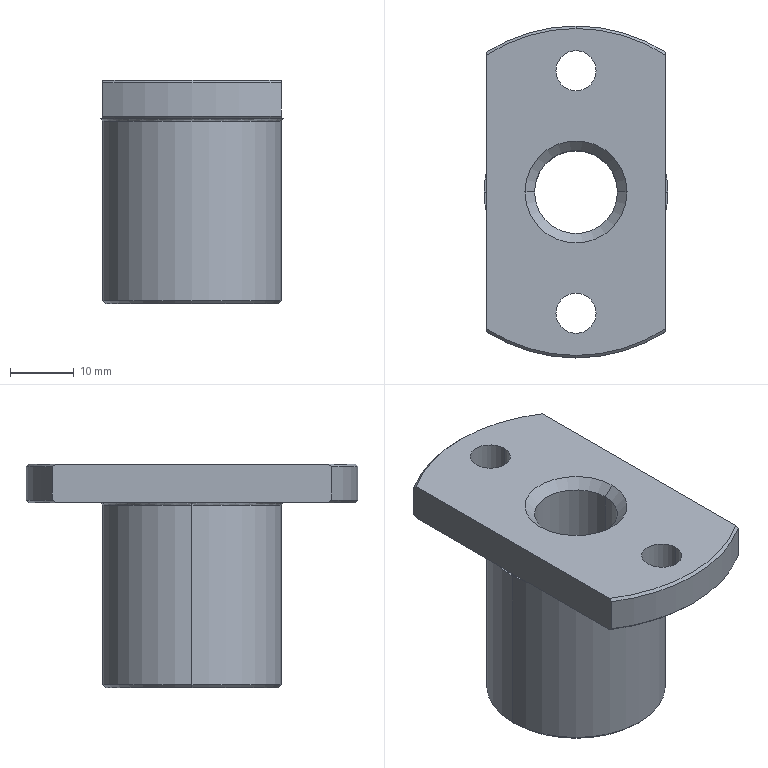Part | SolidWorks | features BaseBody 1 | 1 solid | 31 faces | box 28.8 x 52 x 35 mm | volume 21014 mm3 | cone 11 | cylinder 10 | plane 8 | spline 2 | commonest cylinder face diameters 6.3 x4 13 x2 28 x2 52 x2
STEP:
#1=CARTESIAN_POINT('',(14.4,0.,-6.));
#2=VERTEX_POINT('',#1);
#3=CARTESIAN_POINT('',(14.,3.37,-6.));
#4=VERTEX_POINT('',#3);
#5=CARTESIAN_POINT('',(14.4,0.,-6.));
#6=CARTESIAN_POINT('',(14.4,1.139,-6.));
#7=CARTESIAN_POINT('',(14.267,2.263,-6.));
#8=CARTESIAN_POINT('',(14.,3.37,-6.));
#9=B_SPLINE_CURVE_WITH_KNOTS('',3,(#5,#6,#7,#8),.UNSPECIFIED.,.F.,.F.,(4,4),(0.5,1.),.UNSPECIFIED.);
#10=EDGE_CURVE('',#2,#4,#9,.T.);
#11=ORIENTED_EDGE('',*,*,#10,.F.);
#12=CARTESIAN_POINT('',(14.,0.,-6.4));
#13=VERTEX_POINT('',#12);
#14=CARTESIAN_POINT('',(14.4,0.,-6.4));
#15=DIRECTION('',(0.,-1.,0.));
#16=DIRECTION('',(1.,0.,0.));
#17=AXIS2_PLACEMENT_3D('',#14,#15,#16);
#18=CIRCLE('',#17,0.4);
#19=EDGE_CURVE('',#2,#13,#18,.T.);
#20=ORIENTED_EDGE('',*,*,#19,.T.);
#21=CARTESIAN_POINT('',(-14.,0.,-6.4));
#22=VERTEX_POINT('',#21);
#23=CARTESIAN_POINT('',(0.,0.,-6.4));
#24=DIRECTION('',(0.,0.,-1.));
#25=DIRECTION('',(1.,0.,0.));
#26=AXIS2_PLACEMENT_3D('',#23,#24,#25);
#27=CIRCLE('',#26,14.);
#28=EDGE_CURVE('',#22,#13,#27,.T.);
#29=ORIENTED_EDGE('',*,*,#28,.F.);
#30=CARTESIAN_POINT('',(-14.4,0.,-6.));
#31=VERTEX_POINT('',#30);
#32=CARTESIAN_POINT('',(-14.4,0.,-6.4));
#33=DIRECTION('',(0.,1.,0.));
#34=DIRECTION('',(-1.,0.,0.));
#35=AXIS2_PLACEMENT_3D('',#32,#33,#34);
#36=CIRCLE('',#35,0.4);
#37=EDGE_CURVE('',#31,#22,#36,.T.);
#38=ORIENTED_EDGE('',*,*,#37,.F.);
#39=CARTESIAN_POINT('',(-14.,3.37,-6.));
#40=VERTEX_POINT('',#39);
#41=CARTESIAN_POINT('',(-14.,3.37,-6.));
#42=CARTESIAN_POINT('',(-14.267,2.262,-6.));
#43=CARTESIAN_POINT('',(-14.4,1.139,-6.));
#44=CARTESIAN_POINT('',(-14.4,0.,-6.));
#45=B_SPLINE_CURVE_WITH_KNOTS('',3,(#41,#42,#43,#44),.UNSPECIFIED.,.F.,.F.,(4,4),(0.,0.5),.UNSPECIFIED.);
#46=EDGE_CURVE('',#40,#31,#45,.T.);
#47=ORIENTED_EDGE('',*,*,#46,.F.);
#48=CARTESIAN_POINT('',(14.,3.37,-6.));
#49=CARTESIAN_POINT('',(13.911,3.742,-6.));
#50=CARTESIAN_POINT('',(13.755,4.291,-6.));
#51=CARTESIAN_POINT('',(13.536,4.92,-6.));
#52=CARTESIAN_POINT('',(13.417,5.231,-6.));
#53=CARTESIAN_POINT('',(13.364,5.363,-6.));
#54=CARTESIAN_POINT('',(13.328,5.452,-6.));
#55=CARTESIAN_POINT('',(13.311,5.494,-6.));
#56=CARTESIAN_POINT('',(13.139,5.907,-6.));
#57=CARTESIAN_POINT('',(12.887,6.447,-6.));
#58=CARTESIAN_POINT('',(12.555,7.057,-6.));
#59=CARTESIAN_POINT('',(12.38,7.357,-6.));
#60=CARTESIAN_POINT('',(12.302,7.484,-6.));
#61=CARTESIAN_POINT('',(12.251,7.569,-6.));
#62=CARTESIAN_POINT('',(12.225,7.61,-6.));
#63=CARTESIAN_POINT('',(11.98,8.,-6.));
#64=CARTESIAN_POINT('',(11.632,8.505,-6.));
#65=CARTESIAN_POINT('',(11.19,9.067,-6.));
#66=CARTESIAN_POINT('',(10.993,9.302,-6.));
#67=CARTESIAN_POINT('',(10.86,9.457,-6.));
#68=CARTESIAN_POINT('',(10.794,9.533,-6.));
#69=CARTESIAN_POINT('',(10.169,10.23,-6.));
#70=CARTESIAN_POINT('',(9.565,10.796,-6.));
#71=CARTESIAN_POINT('',(8.585,11.569,-6.));
#72=CARTESIAN_POINT('',(8.08,11.932,-6.));
#73=CARTESIAN_POINT('',(7.465,12.317,-6.));
#74=CARTESIAN_POINT('',(7.196,12.474,-6.));
#75=CARTESIAN_POINT('',(7.015,12.576,-6.));
#76=CARTESIAN_POINT('',(6.923,12.627,-6.));
#77=CARTESIAN_POINT('',(6.472,12.87,-6.));
#78=CARTESIAN_POINT('',(5.921,13.138,-6.));
#79=CARTESIAN_POINT('',(5.259,13.408,-6.));
#80=CARTESIAN_POINT('',(4.924,13.533,-6.));
#81=CARTESIAN_POINT('',(4.779,13.584,-6.));
#82=CARTESIAN_POINT('',(4.683,13.618,-6.));
#83=CARTESIAN_POINT('',(4.633,13.635,-6.));
#84=CARTESIAN_POINT('',(4.208,13.777,-6.));
#85=CARTESIAN_POINT('',(3.636,13.943,-6.));
#86=CARTESIAN_POINT('',(2.959,14.095,-6.));
#87=CARTESIAN_POINT('',(2.618,14.161,-6.));
#88=CARTESIAN_POINT('',(2.471,14.187,-6.));
#89=CARTESIAN_POINT('',(2.373,14.203,-6.));
#90=CARTESIAN_POINT('',(2.322,14.212,-6.));
#91=CARTESIAN_POINT('',(1.521,14.34,-6.));
#92=CARTESIAN_POINT('',(0.7634,14.4,-6.));
#93=CARTESIAN_POINT('',(-0.3817,14.4,-6.));
#94=CARTESIAN_POINT('',(-0.9524,14.377,-6.));
#95=CARTESIAN_POINT('',(-1.615,14.311,-6.));
#96=CARTESIAN_POINT('',(-1.945,14.269,-6.));
#97=CARTESIAN_POINT('',(-2.086,14.248,-6.));
#98=CARTESIAN_POINT('',(-2.181,14.234,-6.));
#99=CARTESIAN_POINT('',(-2.226,14.227,-6.));
#100=CARTESIAN_POINT('',(-2.668,14.156,-6.));
#101=CARTESIAN_POINT('',(-3.252,14.038,-6.));
#102=CARTESIAN_POINT('',(-3.922,13.858,-6.));
#103=CARTESIAN_POINT('',(-4.255,13.758,-6.));
#104=CARTESIAN_POINT('',(-4.397,13.712,-6.));
#105=CARTESIAN_POINT('',(-4.491,13.682,-6.));
#106=CARTESIAN_POINT('',(-4.537,13.667,-6.));
#107=CARTESIAN_POINT('',(-4.974,13.52,-6.));
#108=CARTESIAN_POINT('',(-5.547,13.3,-6.));
#109=CARTESIAN_POINT('',(-6.196,13.002,-6.));
#110=CARTESIAN_POINT('',(-6.47,12.865,-6.));
#111=CARTESIAN_POINT('',(-6.652,12.772,-6.));
#112=CARTESIAN_POINT('',(-6.741,12.725,-6.));
#113=CARTESIAN_POINT('',(-7.565,12.281,-6.));
#114=CARTESIAN_POINT('',(-8.258,11.826,-6.));
#115=CARTESIAN_POINT('',(-9.238,11.054,-6.));
#116=CARTESIAN_POINT('',(-9.71,10.648,-6.));
#117=CARTESIAN_POINT('',(-10.228,10.14,-6.));
#118=CARTESIAN_POINT('',(-10.443,9.916,-6.));
#119=CARTESIAN_POINT('',(-10.585,9.764,-6.));
#120=CARTESIAN_POINT('',(-10.656,9.686,-6.));
#121=CARTESIAN_POINT('',(-10.998,9.305,-6.));
#122=CARTESIAN_POINT('',(-11.387,8.831,-6.));
#123=CARTESIAN_POINT('',(-11.805,8.251,-6.));
#124=CARTESIAN_POINT('',(-12.004,7.955,-6.));
#125=CARTESIAN_POINT('',(-12.088,7.826,-6.));
#126=CARTESIAN_POINT('',(-12.143,7.74,-6.));
#127=CARTESIAN_POINT('',(-12.171,7.695,-6.));
#128=CARTESIAN_POINT('',(-12.409,7.316,-6.));
#129=CARTESIAN_POINT('',(-12.705,6.799,-6.));
#130=CARTESIAN_POINT('',(-13.011,6.176,-6.));
#131=CARTESIAN_POINT('',(-13.155,5.859,-6.));
#132=CARTESIAN_POINT('',(-13.214,5.723,-6.));
#133=CARTESIAN_POINT('',(-13.253,5.631,-6.));
#134=CARTESIAN_POINT('',(-13.273,5.584,-6.));
#135=CARTESIAN_POINT('',(-13.585,4.836,-6.));
#136=CARTESIAN_POINT('',(-13.821,4.112,-6.));
#137=CARTESIAN_POINT('',(-14.,3.37,-6.));
#138=B_SPLINE_CURVE_WITH_KNOTS('',3,(#48,#49,#50,#51,#52,#53,#54,#55,#56,#57,#58,#59,#60,#61,#62,#63,#64,#65,#66,#67,#68,#69,#70,#71,#72,#73,#74,#75,#76,#77,#78,#79,#80,#81,#82,#83,#84,#85,#86,#87,#88,#89,#90,#91,#92,#93,#94,#95,#96,#97,#98,#99,#100,#101,#102,#103,#104,#105,#106,#107,#108,#109,#110,#111,#112,#113,#114,#115,#116,#117,#118,#119,#120,#121,#122,#123,#124,#125,#126,#127,#128,#129,#130,#131,#132,#133,#134,#135,#136,#137),.UNSPECIFIED.,.F.,.F.,(4,1,1,1,2,2,1,1,1,2,2,1,1,2,2,2,1,1,2,2,1,1,1,2,2,1,1,1,2,2,2,1,1,1,2,2,1,1,1,2,2,1,1,2,2,2,1,1,2,2,1,1,1,2,2,1,1,1,2,2,4),(0.,0.03125,0.04688,0.05469,0.05859,0.0625,0.09375,0.1094,0.1172,0.1211,0.125,0.1563,0.1719,0.1797,0.1875,0.25,0.2813,0.2969,0.3047,0.3125,0.3438,0.3594,0.3672,0.3711,0.375,0.4063,0.4219,0.4297,0.4336,0.4375,0.5,0.5313,0.5469,0.5547,0.5586,0.5625,0.5938,0.6094,0.6172,0.6211,0.625,0.6563,0.6719,0.6797,0.6875,0.75,0.7813,0.7969,0.8047,0.8125,0.8438,0.8594,0.8672,0.8711,0.875,0.9063,0.9219,0.9297,0.9336,0.9375,1.),.UNSPECIFIED.);
#139=EDGE_CURVE('',#4,#40,#138,.T.);
#140=ORIENTED_EDGE('',*,*,#139,.F.);
#141=EDGE_LOOP('',(#11,#20,#29,#38,#47,#140));
#142=FACE_OUTER_BOUND('',#141,.T.);
#143=CARTESIAN_POINT('',(-14.4,0.,-6.));
#144=CARTESIAN_POINT('',(-14.4,28.8,-6.));
#145=CARTESIAN_POINT('',(14.4,28.8,-6.));
#146=CARTESIAN_POINT('',(14.4,0.,-6.));
#147=CARTESIAN_POINT('',(-14.166,0.,-6.));
#148=CARTESIAN_POINT('',(-14.166,28.331,-6.));
#149=CARTESIAN_POINT('',(14.166,28.331,-6.));
#150=CARTESIAN_POINT('',(14.166,0.,-6.));
#151=CARTESIAN_POINT('',(-14.,0.,-6.166));
#152=CARTESIAN_POINT('',(-14.,28.,-6.166));
#153=CARTESIAN_POINT('',(14.,28.,-6.166));
#154=CARTESIAN_POINT('',(14.,0.,-6.166));
#155=CARTESIAN_POINT('',(-14.,0.,-6.4));
#156=CARTESIAN_POINT('',(-14.,28.,-6.4));
#157=CARTESIAN_POINT('',(14.,28.,-6.4));
#158=CARTESIAN_POINT('',(14.,0.,-6.4));
#159=(BOUNDED_SURFACE()B_SPLINE_SURFACE(3,3,((#143,#144,#145,#146),(#147,#148,#149,#150),(#151,#152,#153,#154),(#155,#156,#157,#158)),.UNSPECIFIED.,.F.,.F.,.F.)B_SPLINE_SURFACE_WITH_KNOTS((4,4),(4,4),(0.,1.),(0.,1.),.UNSPECIFIED.)GEOMETRIC_REPRESENTATION_ITEM()RATIONAL_B_SPLINE_SURFACE(((1.,0.3333,0.3333,1.),(0.8047,0.2682,0.2682,0.8047),(0.8047,0.2682,0.2682,0.8047),(1.,0.3333,0.3333,1.)))REPRESENTATION_ITEM('')SURFACE());
#160=ADVANCED_FACE('',(#142),#159,.F.);
#161=CARTESIAN_POINT('',(14.,0.,-34.5));
#162=VERTEX_POINT('',#161);
#163=CARTESIAN_POINT('',(-14.,0.,-34.5));
#164=VERTEX_POINT('',#163);
#165=CARTESIAN_POINT('',(0.,0.,-34.5));
#166=DIRECTION('',(0.,0.,1.));
#167=DIRECTION('',(1.,0.,0.));
#168=AXIS2_PLACEMENT_3D('',#165,#166,#167);
#169=CIRCLE('',#168,14.);
#170=EDGE_CURVE('',#162,#164,#169,.T.);
#171=ORIENTED_EDGE('',*,*,#170,.T.);
#172=CARTESIAN_POINT('',(-14.,0.,-35.));
#173=DIRECTION('',(0.,0.,1.));
#174=VECTOR('',#173,1000.);
#175=LINE('',#172,#174);
#176=EDGE_CURVE('',#164,#22,#175,.T.);
#177=ORIENTED_EDGE('',*,*,#176,.T.);
#178=ORIENTED_EDGE('',*,*,#28,.T.);
#179=CARTESIAN_POINT('',(14.,0.,-35.));
#180=DIRECTION('',(0.,0.,1.));
#181=VECTOR('',#180,1000.);
#182=LINE('',#179,#181);
#183=EDGE_CURVE('',#162,#13,#182,.T.);
#184=ORIENTED_EDGE('',*,*,#183,.F.);
#185=EDGE_LOOP('',(#171,#177,#178,#184));
#186=FACE_OUTER_BOUND('',#185,.T.);
#187=CARTESIAN_POINT('',(0.,0.,-35.));
#188=DIRECTION('',(0.,0.,1.));
#189=DIRECTION('',(1.,0.,0.));
#190=AXIS2_PLACEMENT_3D('',#187,#188,#189);
#191=CYLINDRICAL_SURFACE('',#190,14.);
#192=ADVANCED_FACE('',(#186),#191,.T.);
#193=CARTESIAN_POINT('',(13.5,0.,-35.));
#194=VERTEX_POINT('',#193);
#195=CARTESIAN_POINT('',(-13.5,0.,-35.));
#196=VERTEX_POINT('',#195);
#197=CARTESIAN_POINT('',(0.,0.,-35.));
#198=DIRECTION('',(0.,0.,1.));
#199=DIRECTION('',(1.,0.,0.));
#200=AXIS2_PLACEMENT_3D('',#197,#198,#199);
#201=CIRCLE('',#200,13.5);
#202=EDGE_CURVE('',#194,#196,#201,.T.);
#203=ORIENTED_EDGE('',*,*,#202,.T.);
#204=CARTESIAN_POINT('',(-14.,0.,-34.5));
#205=DIRECTION('',(-0.7071,0.,0.7071));
#206=VECTOR('',#205,1000.);
#207=LINE('',#204,#206);
#208=EDGE_CURVE('',#196,#164,#207,.T.);
#209=ORIENTED_EDGE('',*,*,#208,.T.);
#210=ORIENTED_EDGE('',*,*,#170,.F.);
#211=CARTESIAN_POINT('',(14.,0.,-34.5));
#212=DIRECTION('',(0.7071,0.,0.7071));
#213=VECTOR('',#212,1000.);
#214=LINE('',#211,#213);
#215=EDGE_CURVE('',#194,#162,#214,.T.);
#216=ORIENTED_EDGE('',*,*,#215,.F.);
#217=EDGE_LOOP('',(#203,#209,#210,#216));
#218=FACE_OUTER_BOUND('',#217,.T.);
#219=CARTESIAN_POINT('',(0.,0.,-34.5));
#220=DIRECTION('',(0.,0.,1.));
#221=DIRECTION('',(1.,0.,0.));
#222=AXIS2_PLACEMENT_3D('',#219,#220,#221);
#223=CONICAL_SURFACE('',#222,14.,0.7854);
#224=ADVANCED_FACE('',(#218),#223,.T.);
#225=CARTESIAN_POINT('',(3.15,19.,0.));
#226=VERTEX_POINT('',#225);
#227=CARTESIAN_POINT('',(-3.15,19.,0.));
#228=VERTEX_POINT('',#227);
#229=CARTESIAN_POINT('',(0.,19.,0.));
#230=DIRECTION('',(0.,0.,-1.));
#231=DIRECTION('',(-1.,0.,0.));
#232=AXIS2_PLACEMENT_3D('',#229,#230,#231);
#233=CIRCLE('',#232,3.15);
#234=EDGE_CURVE('',#226,#228,#233,.T.);
#235=ORIENTED_EDGE('',*,*,#234,.F.);
#236=CARTESIAN_POINT('',(3.15,19.,-6.));
#237=VERTEX_POINT('',#236);
#238=CARTESIAN_POINT('',(3.15,19.,-6.));
#239=DIRECTION('',(0.,0.,-1.));
#240=VECTOR('',#239,1000.);
#241=LINE('',#238,#240);
#242=EDGE_CURVE('',#226,#237,#241,.T.);
#243=ORIENTED_EDGE('',*,*,#242,.T.);
#244=CARTESIAN_POINT('',(-3.15,19.,-6.));
#245=VERTEX_POINT('',#244);
#246=CARTESIAN_POINT('',(0.,19.,-6.));
#247=DIRECTION('',(0.,0.,-1.));
#248=DIRECTION('',(-1.,0.,0.));
#249=AXIS2_PLACEMENT_3D('',#246,#247,#248);
#250=CIRCLE('',#249,3.15);
#251=EDGE_CURVE('',#237,#245,#250,.T.);
#252=ORIENTED_EDGE('',*,*,#251,.T.);
#253=CARTESIAN_POINT('',(-3.15,19.,-6.));
#254=DIRECTION('',(0.,0.,-1.));
#255=VECTOR('',#254,1000.);
#256=LINE('',#253,#255);
#257=EDGE_CURVE('',#228,#245,#256,.T.);
#258=ORIENTED_EDGE('',*,*,#257,.F.);
#259=EDGE_LOOP('',(#235,#243,#252,#258));
#260=FACE_OUTER_BOUND('',#259,.T.);
#261=CARTESIAN_POINT('',(0.,19.,-6.));
#262=DIRECTION('',(0.,0.,-1.));
#263=DIRECTION('',(-1.,0.,0.));
#264=AXIS2_PLACEMENT_3D('',#261,#262,#263);
#265=CYLINDRICAL_SURFACE('',#264,3.15);
#266=ADVANCED_FACE('',(#260),#265,.F.);
#267=CARTESIAN_POINT('',(3.15,-19.,0.));
#268=VERTEX_POINT('',#267);
#269=CARTESIAN_POINT('',(-3.15,-19.,0.));
#270=VERTEX_POINT('',#269);
#271=CARTESIAN_POINT('',(0.,-19.,0.));
#272=DIRECTION('',(0.,0.,-1.));
#273=DIRECTION('',(-1.,0.,0.));
#274=AXIS2_PLACEMENT_3D('',#271,#272,#273);
#275=CIRCLE('',#274,3.15);
#276=EDGE_CURVE('',#268,#270,#275,.T.);
#277=ORIENTED_EDGE('',*,*,#276,.F.);
#278=CARTESIAN_POINT('',(3.15,-19.,-6.));
#279=VERTEX_POINT('',#278);
#280=CARTESIAN_POINT('',(3.15,-19.,-6.));
#281=DIRECTION('',(0.,0.,-1.));
#282=VECTOR('',#281,1000.);
#283=LINE('',#280,#282);
#284=EDGE_CURVE('',#268,#279,#283,.T.);
#285=ORIENTED_EDGE('',*,*,#284,.T.);
#286=CARTESIAN_POINT('',(-3.15,-19.,-6.));
#287=VERTEX_POINT('',#286);
#288=CARTESIAN_POINT('',(0.,-19.,-6.));
#289=DIRECTION('',(0.,0.,-1.));
#290=DIRECTION('',(-1.,0.,0.));
#291=AXIS2_PLACEMENT_3D('',#288,#289,#290);
#292=CIRCLE('',#291,3.15);
#293=EDGE_CURVE('',#279,#287,#292,.T.);
#294=ORIENTED_EDGE('',*,*,#293,.T.);
#295=CARTESIAN_POINT('',(-3.15,-19.,-6.));
#296=DIRECTION('',(0.,0.,-1.));
#297=VECTOR('',#296,1000.);
#298=LINE('',#295,#297);
#299=EDGE_CURVE('',#270,#287,#298,.T.);
#300=ORIENTED_EDGE('',*,*,#299,.F.);
#301=EDGE_LOOP('',(#277,#285,#294,#300));
#302=FACE_OUTER_BOUND('',#301,.T.);
#303=CARTESIAN_POINT('',(0.,-19.,-6.));
#304=DIRECTION('',(0.,0.,-1.));
#305=DIRECTION('',(-1.,0.,0.));
#306=AXIS2_PLACEMENT_3D('',#303,#304,#305);
#307=CYLINDRICAL_SURFACE('',#306,3.15);
#308=ADVANCED_FACE('',(#302),#307,.F.);
#309=CARTESIAN_POINT('',(6.5,0.,-33.5));
#310=VERTEX_POINT('',#309);
#311=CARTESIAN_POINT('',(-6.5,0.,-33.5));
#312=VERTEX_POINT('',#311);
#313=CARTESIAN_POINT('',(0.,0.,-33.5));
#314=DIRECTION('',(0.,0.,-1.));
#315=DIRECTION('',(-1.,0.,0.));
#316=AXIS2_PLACEMENT_3D('',#313,#314,#315);
#317=CIRCLE('',#316,6.5);
#318=EDGE_CURVE('',#310,#312,#317,.T.);
#319=ORIENTED_EDGE('',*,*,#318,.F.);
#320=CARTESIAN_POINT('',(8.,0.,-35.));
#321=VERTEX_POINT('',#320);
#322=CARTESIAN_POINT('',(8.,0.,-35.));
#323=DIRECTION('',(0.7071,0.,-0.7071));
#324=VECTOR('',#323,1000.);
#325=LINE('',#322,#324);
#326=EDGE_CURVE('',#310,#321,#325,.T.);
#327=ORIENTED_EDGE('',*,*,#326,.T.);
#328=CARTESIAN_POINT('',(-8.,0.,-35.));
#329=VERTEX_POINT('',#328);
#330=CARTESIAN_POINT('',(0.,0.,-35.));
#331=DIRECTION('',(0.,0.,-1.));
#332=DIRECTION('',(-1.,0.,0.));
#333=AXIS2_PLACEMENT_3D('',#330,#331,#332);
#334=CIRCLE('',#333,8.);
#335=EDGE_CURVE('',#321,#329,#334,.T.);
#336=ORIENTED_EDGE('',*,*,#335,.T.);
#337=CARTESIAN_POINT('',(-8.,0.,-35.));
#338=DIRECTION('',(-0.7071,0.,-0.7071));
#339=VECTOR('',#338,1000.);
#340=LINE('',#337,#339);
#341=EDGE_CURVE('',#312,#329,#340,.T.);
#342=ORIENTED_EDGE('',*,*,#341,.F.);
#343=EDGE_LOOP('',(#319,#327,#336,#342));
#344=FACE_OUTER_BOUND('',#343,.T.);
#345=CARTESIAN_POINT('',(0.,0.,-35.));
#346=DIRECTION('',(0.,0.,-1.));
#347=DIRECTION('',(-1.,0.,0.));
#348=AXIS2_PLACEMENT_3D('',#345,#346,#347);
#349=CONICAL_SURFACE('',#348,8.,0.7854);
#350=ADVANCED_FACE('',(#344),#349,.F.);
#351=ORIENTED_EDGE('',*,*,#318,.T.);
#352=CARTESIAN_POINT('',(-6.5,0.,-1.5));
#353=VERTEX_POINT('',#352);
#354=CARTESIAN_POINT('',(-6.5,0.,-35.));
#355=DIRECTION('',(0.,0.,1.));
#356=VECTOR('',#355,1000.);
#357=LINE('',#354,#356);
#358=EDGE_CURVE('',#312,#353,#357,.T.);
#359=ORIENTED_EDGE('',*,*,#358,.T.);
#360=CARTESIAN_POINT('',(6.5,0.,-1.5));
#361=VERTEX_POINT('',#360);
#362=CARTESIAN_POINT('',(0.,0.,-1.5));
#363=DIRECTION('',(0.,0.,-1.));
#364=DIRECTION('',(1.,0.,0.));
#365=AXIS2_PLACEMENT_3D('',#362,#363,#364);
#366=CIRCLE('',#365,6.5);
#367=EDGE_CURVE('',#361,#353,#366,.T.);
#368=ORIENTED_EDGE('',*,*,#367,.F.);
#369=CARTESIAN_POINT('',(6.5,0.,-35.));
#370=DIRECTION('',(0.,0.,1.));
#371=VECTOR('',#370,1000.);
#372=LINE('',#369,#371);
#373=EDGE_CURVE('',#310,#361,#372,.T.);
#374=ORIENTED_EDGE('',*,*,#373,.F.);
#375=EDGE_LOOP('',(#351,#359,#368,#374));
#376=FACE_OUTER_BOUND('',#375,.T.);
#377=CARTESIAN_POINT('',(0.,0.,-35.));
#378=DIRECTION('',(0.,0.,1.));
#379=DIRECTION('',(1.,0.,0.));
#380=AXIS2_PLACEMENT_3D('',#377,#378,#379);
#381=CYLINDRICAL_SURFACE('',#380,6.5);
#382=ADVANCED_FACE('',(#376),#381,.F.);
#383=ORIENTED_EDGE('',*,*,#367,.T.);
#384=CARTESIAN_POINT('',(-8.,0.,0.));
#385=VERTEX_POINT('',#384);
#386=CARTESIAN_POINT('',(-8.,0.,0.));
#387=DIRECTION('',(-0.7071,0.,0.7071));
#388=VECTOR('',#387,1000.);
#389=LINE('',#386,#388);
#390=EDGE_CURVE('',#353,#385,#389,.T.);
#391=ORIENTED_EDGE('',*,*,#390,.T.);
#392=CARTESIAN_POINT('',(8.,0.,0.));
#393=VERTEX_POINT('',#392);
#394=CARTESIAN_POINT('',(0.,0.,0.));
#395=DIRECTION('',(0.,0.,-1.));
#396=DIRECTION('',(1.,0.,0.));
#397=AXIS2_PLACEMENT_3D('',#394,#395,#396);
#398=CIRCLE('',#397,8.);
#399=EDGE_CURVE('',#393,#385,#398,.T.);
#400=ORIENTED_EDGE('',*,*,#399,.F.);
#401=CARTESIAN_POINT('',(8.,0.,0.));
#402=DIRECTION('',(0.7071,0.,0.7071));
#403=VECTOR('',#402,1000.);
#404=LINE('',#401,#403);
#405=EDGE_CURVE('',#361,#393,#404,.T.);
#406=ORIENTED_EDGE('',*,*,#405,.F.);
#407=EDGE_LOOP('',(#383,#391,#400,#406));
#408=FACE_OUTER_BOUND('',#407,.T.);
#409=CARTESIAN_POINT('',(0.,0.,0.));
#410=DIRECTION('',(0.,0.,1.));
#411=DIRECTION('',(1.,0.,0.));
#412=AXIS2_PLACEMENT_3D('',#409,#410,#411);
#413=CONICAL_SURFACE('',#412,8.,0.7854);
#414=ADVANCED_FACE('',(#408),#413,.F.);
#415=CARTESIAN_POINT('',(0.,25.6,0.));
#416=VERTEX_POINT('',#415);
#417=CARTESIAN_POINT('',(-14.,21.433,0.));
#418=VERTEX_POINT('',#417);
#419=CARTESIAN_POINT('',(0.,0.,0.));
#420=DIRECTION('',(0.,0.,1.));
#421=DIRECTION('',(0.,1.,0.));
#422=AXIS2_PLACEMENT_3D('',#419,#420,#421);
#423=CIRCLE('',#422,25.6);
#424=EDGE_CURVE('',#416,#418,#423,.T.);
#425=ORIENTED_EDGE('',*,*,#424,.F.);
#426=CARTESIAN_POINT('',(0.,26.,-0.4));
#427=VERTEX_POINT('',#426);
#428=CARTESIAN_POINT('',(0.,26.,-0.4));
#429=DIRECTION('',(0.,0.7071,-0.7071));
#430=VECTOR('',#429,1000.);
#431=LINE('',#428,#430);
#432=EDGE_CURVE('',#416,#427,#431,.T.);
#433=ORIENTED_EDGE('',*,*,#432,.T.);
#434=CARTESIAN_POINT('',(-14.,21.909,-0.4));
#435=VERTEX_POINT('',#434);
#436=CARTESIAN_POINT('',(0.,0.,-0.4));
#437=DIRECTION('',(0.,0.,-1.));
#438=DIRECTION('',(-1.,0.,0.));
#439=AXIS2_PLACEMENT_3D('',#436,#437,#438);
#440=CIRCLE('',#439,26.);
#441=EDGE_CURVE('',#435,#427,#440,.T.);
#442=ORIENTED_EDGE('',*,*,#441,.F.);
#443=CARTESIAN_POINT('',(-14.,21.909,-0.4));
#444=CARTESIAN_POINT('',(-14.,21.75,-0.2664));
#445=CARTESIAN_POINT('',(-14.,21.592,-0.1331));
#446=CARTESIAN_POINT('',(-14.,21.433,0.));
#447=B_SPLINE_CURVE_WITH_KNOTS('',3,(#443,#444,#445,#446),.UNSPECIFIED.,.F.,.F.,(4,4),(0.,0.0006219),.UNSPECIFIED.);
#448=EDGE_CURVE('',#435,#418,#447,.T.);
#449=ORIENTED_EDGE('',*,*,#448,.T.);
#450=EDGE_LOOP('',(#425,#433,#442,#449));
#451=FACE_OUTER_BOUND('',#450,.T.);
#452=CARTESIAN_POINT('',(0.,0.,-0.4));
#453=DIRECTION('',(0.,0.,-1.));
#454=DIRECTION('',(0.,1.,0.));
#455=AXIS2_PLACEMENT_3D('',#452,#453,#454);
#456=CONICAL_SURFACE('',#455,26.,0.7854);
#457=ADVANCED_FACE('',(#451),#456,.T.);
#458=ORIENTED_EDGE('',*,*,#176,.F.);
#459=CARTESIAN_POINT('',(0.,0.,-34.5));
#460=DIRECTION('',(0.,0.,1.));
#461=DIRECTION('',(1.,0.,0.));
#462=AXIS2_PLACEMENT_3D('',#459,#460,#461);
#463=CIRCLE('',#462,14.);
#464=EDGE_CURVE('',#164,#162,#463,.T.);
#465=ORIENTED_EDGE('',*,*,#464,.T.);
#466=ORIENTED_EDGE('',*,*,#183,.T.);
#467=CARTESIAN_POINT('',(0.,0.,-6.4));
#468=DIRECTION('',(0.,0.,-1.));
#469=DIRECTION('',(1.,0.,0.));
#470=AXIS2_PLACEMENT_3D('',#467,#468,#469);
#471=CIRCLE('',#470,14.);
#472=EDGE_CURVE('',#13,#22,#471,.T.);
#473=ORIENTED_EDGE('',*,*,#472,.T.);
#474=EDGE_LOOP('',(#458,#465,#466,#473));
#475=FACE_OUTER_BOUND('',#474,.T.);
#476=CARTESIAN_POINT('',(0.,0.,-35.));
#477=DIRECTION('',(0.,0.,1.));
#478=DIRECTION('',(1.,0.,0.));
#479=AXIS2_PLACEMENT_3D('',#476,#477,#478);
#480=CYLINDRICAL_SURFACE('',#479,14.);
#481=ADVANCED_FACE('',(#475),#480,.T.);
#482=ORIENTED_EDGE('',*,*,#19,.F.);
#483=CARTESIAN_POINT('',(14.,-3.37,-6.));
#484=VERTEX_POINT('',#483);
#485=CARTESIAN_POINT('',(14.,-3.37,-6.));
#486=CARTESIAN_POINT('',(14.267,-2.262,-6.));
#487=CARTESIAN_POINT('',(14.4,-1.139,-6.));
#488=CARTESIAN_POINT('',(14.4,0.,-6.));
#489=B_SPLINE_CURVE_WITH_KNOTS('',3,(#485,#486,#487,#488),.UNSPECIFIED.,.F.,.F.,(4,4),(0.,0.5),.UNSPECIFIED.);
#490=EDGE_CURVE('',#484,#2,#489,.T.);
#491=ORIENTED_EDGE('',*,*,#490,.F.);
#492=CARTESIAN_POINT('',(-14.,-3.37,-6.));
#493=VERTEX_POINT('',#492);
#494=CARTESIAN_POINT('',(-14.,-3.37,-6.));
#495=CARTESIAN_POINT('',(-13.911,-3.742,-6.));
#496=CARTESIAN_POINT('',(-13.755,-4.291,-6.));
#497=CARTESIAN_POINT('',(-13.536,-4.92,-6.));
#498=CARTESIAN_POINT('',(-13.417,-5.231,-6.));
#499=CARTESIAN_POINT('',(-13.364,-5.363,-6.));
#500=CARTESIAN_POINT('',(-13.328,-5.452,-6.));
#501=CARTESIAN_POINT('',(-13.311,-5.494,-6.));
#502=CARTESIAN_POINT('',(-13.139,-5.907,-6.));
#503=CARTESIAN_POINT('',(-12.887,-6.447,-6.));
#504=CARTESIAN_POINT('',(-12.555,-7.057,-6.));
#505=CARTESIAN_POINT('',(-12.38,-7.357,-6.));
#506=CARTESIAN_POINT('',(-12.302,-7.484,-6.));
#507=CARTESIAN_POINT('',(-12.251,-7.569,-6.));
#508=CARTESIAN_POINT('',(-12.225,-7.61,-6.));
#509=CARTESIAN_POINT('',(-11.98,-8.,-6.));
#510=CARTESIAN_POINT('',(-11.632,-8.505,-6.));
#511=CARTESIAN_POINT('',(-11.19,-9.067,-6.));
#512=CARTESIAN_POINT('',(-10.993,-9.302,-6.));
#513=CARTESIAN_POINT('',(-10.86,-9.457,-6.));
#514=CARTESIAN_POINT('',(-10.794,-9.533,-6.));
#515=CARTESIAN_POINT('',(-10.169,-10.23,-6.));
#516=CARTESIAN_POINT('',(-9.565,-10.796,-6.));
#517=CARTESIAN_POINT('',(-8.585,-11.569,-6.));
#518=CARTESIAN_POINT('',(-8.08,-11.932,-6.));
#519=CARTESIAN_POINT('',(-7.465,-12.317,-6.));
#520=CARTESIAN_POINT('',(-7.196,-12.474,-6.));
#521=CARTESIAN_POINT('',(-7.015,-12.576,-6.));
#522=CARTESIAN_POINT('',(-6.923,-12.627,-6.));
#523=CARTESIAN_POINT('',(-6.472,-12.87,-6.));
#524=CARTESIAN_POINT('',(-5.921,-13.138,-6.));
#525=CARTESIAN_POINT('',(-5.259,-13.408,-6.));
#526=CARTESIAN_POINT('',(-4.924,-13.533,-6.));
#527=CARTESIAN_POINT('',(-4.779,-13.584,-6.));
#528=CARTESIAN_POINT('',(-4.683,-13.618,-6.));
#529=CARTESIAN_POINT('',(-4.633,-13.635,-6.));
#530=CARTESIAN_POINT('',(-4.208,-13.777,-6.));
#531=CARTESIAN_POINT('',(-3.636,-13.943,-6.));
#532=CARTESIAN_POINT('',(-2.959,-14.095,-6.));
#533=CARTESIAN_POINT('',(-2.618,-14.161,-6.));
#534=CARTESIAN_POINT('',(-2.471,-14.187,-6.));
#535=CARTESIAN_POINT('',(-2.373,-14.203,-6.));
#536=CARTESIAN_POINT('',(-2.322,-14.212,-6.));
#537=CARTESIAN_POINT('',(-1.521,-14.34,-6.));
#538=CARTESIAN_POINT('',(-0.7634,-14.4,-6.));
#539=CARTESIAN_POINT('',(0.3817,-14.4,-6.));
#540=CARTESIAN_POINT('',(0.9524,-14.377,-6.));
#541=CARTESIAN_POINT('',(1.615,-14.311,-6.));
#542=CARTESIAN_POINT('',(1.945,-14.269,-6.));
#543=CARTESIAN_POINT('',(2.086,-14.248,-6.));
#544=CARTESIAN_POINT('',(2.181,-14.234,-6.));
#545=CARTESIAN_POINT('',(2.226,-14.227,-6.));
#546=CARTESIAN_POINT('',(2.668,-14.156,-6.));
#547=CARTESIAN_POINT('',(3.252,-14.038,-6.));
#548=CARTESIAN_POINT('',(3.922,-13.858,-6.));
#549=CARTESIAN_POINT('',(4.255,-13.758,-6.));
#550=CARTESIAN_POINT('',(4.397,-13.712,-6.));
#551=CARTESIAN_POINT('',(4.491,-13.682,-6.));
#552=CARTESIAN_POINT('',(4.537,-13.667,-6.));
#553=CARTESIAN_POINT('',(4.974,-13.52,-6.));
#554=CARTESIAN_POINT('',(5.547,-13.3,-6.));
#555=CARTESIAN_POINT('',(6.196,-13.002,-6.));
#556=CARTESIAN_POINT('',(6.47,-12.865,-6.));
#557=CARTESIAN_POINT('',(6.652,-12.772,-6.));
#558=CARTESIAN_POINT('',(6.741,-12.725,-6.));
#559=CARTESIAN_POINT('',(7.565,-12.281,-6.));
#560=CARTESIAN_POINT('',(8.258,-11.826,-6.));
#561=CARTESIAN_POINT('',(9.238,-11.054,-6.));
#562=CARTESIAN_POINT('',(9.71,-10.648,-6.));
#563=CARTESIAN_POINT('',(10.228,-10.14,-6.));
#564=CARTESIAN_POINT('',(10.443,-9.916,-6.));
#565=CARTESIAN_POINT('',(10.585,-9.764,-6.));
#566=CARTESIAN_POINT('',(10.656,-9.686,-6.));
#567=CARTESIAN_POINT('',(10.998,-9.305,-6.));
#568=CARTESIAN_POINT('',(11.387,-8.831,-6.));
#569=CARTESIAN_POINT('',(11.805,-8.251,-6.));
#570=CARTESIAN_POINT('',(12.004,-7.955,-6.));
#571=CARTESIAN_POINT('',(12.088,-7.826,-6.));
#572=CARTESIAN_POINT('',(12.143,-7.74,-6.));
#573=CARTESIAN_POINT('',(12.171,-7.695,-6.));
#574=CARTESIAN_POINT('',(12.409,-7.316,-6.));
#575=CARTESIAN_POINT('',(12.705,-6.799,-6.));
#576=CARTESIAN_POINT('',(13.011,-6.176,-6.));
#577=CARTESIAN_POINT('',(13.155,-5.859,-6.));
#578=CARTESIAN_POINT('',(13.214,-5.723,-6.));
#579=CARTESIAN_POINT('',(13.253,-5.631,-6.));
#580=CARTESIAN_POINT('',(13.273,-5.584,-6.));
#581=CARTESIAN_POINT('',(13.585,-4.836,-6.));
#582=CARTESIAN_POINT('',(13.821,-4.112,-6.));
#583=CARTESIAN_POINT('',(14.,-3.37,-6.));
#584=B_SPLINE_CURVE_WITH_KNOTS('',3,(#494,#495,#496,#497,#498,#499,#500,#501,#502,#503,#504,#505,#506,#507,#508,#509,#510,#511,#512,#513,#514,#515,#516,#517,#518,#519,#520,#521,#522,#523,#524,#525,#526,#527,#528,#529,#530,#531,#532,#533,#534,#535,#536,#537,#538,#539,#540,#541,#542,#543,#544,#545,#546,#547,#548,#549,#550,#551,#552,#553,#554,#555,#556,#557,#558,#559,#560,#561,#562,#563,#564,#565,#566,#567,#568,#569,#570,#571,#572,#573,#574,#575,#576,#577,#578,#579,#580,#581,#582,#583),.UNSPECIFIED.,.F.,.F.,(4,1,1,1,2,2,1,1,1,2,2,1,1,2,2,2,1,1,2,2,1,1,1,2,2,1,1,1,2,2,2,1,1,1,2,2,1,1,1,2,2,1,1,2,2,2,1,1,2,2,1,1,1,2,2,1,1,1,2,2,4),(0.,0.03125,0.04687,0.05469,0.05859,0.0625,0.09375,0.1094,0.1172,0.1211,0.125,0.1562,0.1719,0.1797,0.1875,0.25,0.2812,0.2969,0.3047,0.3125,0.3437,0.3594,0.3672,0.3711,0.375,0.4062,0.4219,0.4297,0.4336,0.4375,0.5,0.5313,0.5469,0.5547,0.5586,0.5625,0.5938,0.6094,0.6172,0.6211,0.625,0.6563,0.6719,0.6797,0.6875,0.75,0.7813,0.7969,0.8047,0.8125,0.8438,0.8594,0.8672,0.8711,0.875,0.9063,0.9219,0.9297,0.9336,0.9375,1.),.UNSPECIFIED.);
#585=EDGE_CURVE('',#493,#484,#584,.T.);
#586=ORIENTED_EDGE('',*,*,#585,.F.);
#587=CARTESIAN_POINT('',(-14.4,0.,-6.));
#588=CARTESIAN_POINT('',(-14.4,-1.139,-6.));
#589=CARTESIAN_POINT('',(-14.267,-2.263,-6.));
#590=CARTESIAN_POINT('',(-14.,-3.37,-6.));
#591=B_SPLINE_CURVE_WITH_KNOTS('',3,(#587,#588,#589,#590),.UNSPECIFIED.,.F.,.F.,(4,4),(0.5,1.),.UNSPECIFIED.);
#592=EDGE_CURVE('',#31,#493,#591,.T.);
#593=ORIENTED_EDGE('',*,*,#592,.F.);
#594=ORIENTED_EDGE('',*,*,#37,.T.);
#595=ORIENTED_EDGE('',*,*,#472,.F.);
#596=EDGE_LOOP('',(#482,#491,#586,#593,#594,#595));
#597=FACE_OUTER_BOUND('',#596,.T.);
#598=CARTESIAN_POINT('',(14.4,0.,-6.));
#599=CARTESIAN_POINT('',(14.4,-28.8,-6.));
#600=CARTESIAN_POINT('',(-14.4,-28.8,-6.));
#601=CARTESIAN_POINT('',(-14.4,0.,-6.));
#602=CARTESIAN_POINT('',(14.166,0.,-6.));
#603=CARTESIAN_POINT('',(14.166,-28.331,-6.));
#604=CARTESIAN_POINT('',(-14.166,-28.331,-6.));
#605=CARTESIAN_POINT('',(-14.166,0.,-6.));
#606=CARTESIAN_POINT('',(14.,0.,-6.166));
#607=CARTESIAN_POINT('',(14.,-28.,-6.166));
#608=CARTESIAN_POINT('',(-14.,-28.,-6.166));
#609=CARTESIAN_POINT('',(-14.,0.,-6.166));
#610=CARTESIAN_POINT('',(14.,0.,-6.4));
#611=CARTESIAN_POINT('',(14.,-28.,-6.4));
#612=CARTESIAN_POINT('',(-14.,-28.,-6.4));
#613=CARTESIAN_POINT('',(-14.,0.,-6.4));
#614=(BOUNDED_SURFACE()B_SPLINE_SURFACE(3,3,((#598,#599,#600,#601),(#602,#603,#604,#605),(#606,#607,#608,#609),(#610,#611,#612,#613)),.UNSPECIFIED.,.F.,.F.,.F.)B_SPLINE_SURFACE_WITH_KNOTS((4,4),(4,4),(0.,1.),(0.,1.),.UNSPECIFIED.)GEOMETRIC_REPRESENTATION_ITEM()RATIONAL_B_SPLINE_SURFACE(((1.,0.3333,0.3333,1.),(0.8047,0.2682,0.2682,0.8047),(0.8047,0.2682,0.2682,0.8047),(1.,0.3333,0.3333,1.)))REPRESENTATION_ITEM('')SURFACE());
#615=ADVANCED_FACE('',(#597),#614,.F.);
#616=ORIENTED_EDGE('',*,*,#208,.F.);
#617=CARTESIAN_POINT('',(0.,0.,-35.));
#618=DIRECTION('',(0.,0.,1.));
#619=DIRECTION('',(1.,0.,0.));
#620=AXIS2_PLACEMENT_3D('',#617,#618,#619);
#621=CIRCLE('',#620,13.5);
#622=EDGE_CURVE('',#196,#194,#621,.T.);
#623=ORIENTED_EDGE('',*,*,#622,.T.);
#624=ORIENTED_EDGE('',*,*,#215,.T.);
#625=ORIENTED_EDGE('',*,*,#464,.F.);
#626=EDGE_LOOP('',(#616,#623,#624,#625));
#627=FACE_OUTER_BOUND('',#626,.T.);
#628=CARTESIAN_POINT('',(0.,0.,-34.5));
#629=DIRECTION('',(0.,0.,1.));
#630=DIRECTION('',(1.,0.,0.));
#631=AXIS2_PLACEMENT_3D('',#628,#629,#630);
#632=CONICAL_SURFACE('',#631,14.,0.7854);
#633=ADVANCED_FACE('',(#627),#632,.T.);
#634=CARTESIAN_POINT('',(-14.,0.,-6.));
#635=DIRECTION('',(0.,-1.,0.));
#636=VECTOR('',#635,1000.);
#637=LINE('',#634,#636);
#638=EDGE_CURVE('',#40,#493,#637,.T.);
#639=ORIENTED_EDGE('',*,*,#638,.F.);
#640=ORIENTED_EDGE('',*,*,#46,.T.);
#641=ORIENTED_EDGE('',*,*,#592,.T.);
#642=EDGE_LOOP('',(#639,#640,#641));
#643=FACE_OUTER_BOUND('',#642,.T.);
#644=CARTESIAN_POINT('',(0.,0.,-6.));
#645=DIRECTION('',(0.,0.,-1.));
#646=DIRECTION('',(-1.,0.,0.));
#647=AXIS2_PLACEMENT_3D('',#644,#645,#646);
#648=PLANE('',#647);
#649=ADVANCED_FACE('',(#643),#648,.F.);
#650=CARTESIAN_POINT('',(14.,21.433,-6.));
#651=VERTEX_POINT('',#650);
#652=CARTESIAN_POINT('',(14.,0.,-6.));
#653=DIRECTION('',(0.,1.,0.));
#654=VECTOR('',#653,1000.);
#655=LINE('',#652,#654);
#656=EDGE_CURVE('',#4,#651,#655,.T.);
#657=ORIENTED_EDGE('',*,*,#656,.F.);
#658=ORIENTED_EDGE('',*,*,#139,.T.);
#659=CARTESIAN_POINT('',(-14.,21.433,-6.));
#660=VERTEX_POINT('',#659);
#661=CARTESIAN_POINT('',(-14.,0.,-6.));
#662=DIRECTION('',(0.,-1.,0.));
#663=VECTOR('',#662,1000.);
#664=LINE('',#661,#663);
#665=EDGE_CURVE('',#660,#40,#664,.T.);
#666=ORIENTED_EDGE('',*,*,#665,.F.);
#667=CARTESIAN_POINT('',(0.,0.,-6.));
#668=DIRECTION('',(0.,0.,1.));
#669=DIRECTION('',(1.,0.,0.));
#670=AXIS2_PLACEMENT_3D('',#667,#668,#669);
#671=CIRCLE('',#670,25.6);
#672=EDGE_CURVE('',#651,#660,#671,.T.);
#673=ORIENTED_EDGE('',*,*,#672,.F.);
#674=EDGE_LOOP('',(#657,#658,#666,#673));
#675=FACE_OUTER_BOUND('',#674,.T.);
#676=CARTESIAN_POINT('',(0.,19.,-6.));
#677=DIRECTION('',(0.,0.,-1.));
#678=DIRECTION('',(-1.,0.,0.));
#679=AXIS2_PLACEMENT_3D('',#676,#677,#678);
#680=CIRCLE('',#679,3.15);
#681=EDGE_CURVE('',#245,#237,#680,.T.);
#682=ORIENTED_EDGE('',*,*,#681,.F.);
#683=ORIENTED_EDGE('',*,*,#251,.F.);
#684=EDGE_LOOP('',(#682,#683));
#685=FACE_BOUND('',#684,.T.);
#686=CARTESIAN_POINT('',(0.,0.,-6.));
#687=DIRECTION('',(0.,0.,1.));
#688=DIRECTION('',(1.,0.,0.));
#689=AXIS2_PLACEMENT_3D('',#686,#687,#688);
#690=PLANE('',#689);
#691=ADVANCED_FACE('',(#675,#685),#690,.F.);
#692=CARTESIAN_POINT('',(14.,0.,-6.));
#693=DIRECTION('',(0.,1.,0.));
#694=VECTOR('',#693,1000.);
#695=LINE('',#692,#694);
#696=EDGE_CURVE('',#484,#4,#695,.T.);
#697=ORIENTED_EDGE('',*,*,#696,.F.);
#698=ORIENTED_EDGE('',*,*,#490,.T.);
#699=ORIENTED_EDGE('',*,*,#10,.T.);
#700=EDGE_LOOP('',(#697,#698,#699));
#701=FACE_OUTER_BOUND('',#700,.T.);
#702=CARTESIAN_POINT('',(0.,0.,-6.));
#703=DIRECTION('',(0.,0.,-1.));
#704=DIRECTION('',(-1.,0.,0.));
#705=AXIS2_PLACEMENT_3D('',#702,#703,#704);
#706=PLANE('',#705);
#707=ADVANCED_FACE('',(#701),#706,.F.);
#708=CARTESIAN_POINT('',(-14.,-21.433,-6.));
#709=VERTEX_POINT('',#708);
#710=CARTESIAN_POINT('',(14.,-21.433,-6.));
#711=VERTEX_POINT('',#710);
#712=CARTESIAN_POINT('',(0.,0.,-6.));
#713=DIRECTION('',(0.,0.,1.));
#714=DIRECTION('',(1.,0.,0.));
#715=AXIS2_PLACEMENT_3D('',#712,#713,#714);
#716=CIRCLE('',#715,25.6);
#717=EDGE_CURVE('',#709,#711,#716,.T.);
#718=ORIENTED_EDGE('',*,*,#717,.F.);
#719=CARTESIAN_POINT('',(-14.,0.,-6.));
#720=DIRECTION('',(0.,-1.,0.));
#721=VECTOR('',#720,1000.);
#722=LINE('',#719,#721);
#723=EDGE_CURVE('',#493,#709,#722,.T.);
#724=ORIENTED_EDGE('',*,*,#723,.F.);
#725=ORIENTED_EDGE('',*,*,#585,.T.);
#726=CARTESIAN_POINT('',(14.,0.,-6.));
#727=DIRECTION('',(0.,1.,0.));
#728=VECTOR('',#727,1000.);
#729=LINE('',#726,#728);
#730=EDGE_CURVE('',#711,#484,#729,.T.);
#731=ORIENTED_EDGE('',*,*,#730,.F.);
#732=EDGE_LOOP('',(#718,#724,#725,#731));
#733=FACE_OUTER_BOUND('',#732,.T.);
#734=CARTESIAN_POINT('',(0.,-19.,-6.));
#735=DIRECTION('',(0.,0.,-1.));
#736=DIRECTION('',(-1.,0.,0.));
#737=AXIS2_PLACEMENT_3D('',#734,#735,#736);
#738=CIRCLE('',#737,3.15);
#739=EDGE_CURVE('',#287,#279,#738,.T.);
#740=ORIENTED_EDGE('',*,*,#739,.F.);
#741=ORIENTED_EDGE('',*,*,#293,.F.);
#742=EDGE_LOOP('',(#740,#741));
#743=FACE_BOUND('',#742,.T.);
#744=CARTESIAN_POINT('',(0.,0.,-6.));
#745=DIRECTION('',(0.,0.,1.));
#746=DIRECTION('',(1.,0.,0.));
#747=AXIS2_PLACEMENT_3D('',#744,#745,#746);
#748=PLANE('',#747);
#749=ADVANCED_FACE('',(#733,#743),#748,.F.);
#750=ORIENTED_EDGE('',*,*,#202,.F.);
#751=ORIENTED_EDGE('',*,*,#622,.F.);
#752=EDGE_LOOP('',(#750,#751));
#753=FACE_OUTER_BOUND('',#752,.T.);
#754=CARTESIAN_POINT('',(0.,0.,-35.));
#755=DIRECTION('',(0.,0.,-1.));
#756=DIRECTION('',(-1.,0.,0.));
#757=AXIS2_PLACEMENT_3D('',#754,#755,#756);
#758=CIRCLE('',#757,8.);
#759=EDGE_CURVE('',#329,#321,#758,.T.);
#760=ORIENTED_EDGE('',*,*,#759,.F.);
#761=ORIENTED_EDGE('',*,*,#335,.F.);
#762=EDGE_LOOP('',(#760,#761));
#763=FACE_BOUND('',#762,.T.);
#764=CARTESIAN_POINT('',(0.,13.5,-35.));
#765=DIRECTION('',(0.,0.,1.));
#766=DIRECTION('',(1.,0.,0.));
#767=AXIS2_PLACEMENT_3D('',#764,#765,#766);
#768=PLANE('',#767);
#769=ADVANCED_FACE('',(#753,#763),#768,.F.);
#770=CARTESIAN_POINT('',(-14.,-21.433,0.));
#771=VERTEX_POINT('',#770);
#772=CARTESIAN_POINT('',(-14.,-21.909,-0.4));
#773=VERTEX_POINT('',#772);
#774=CARTESIAN_POINT('',(-14.,-21.433,0.));
#775=CARTESIAN_POINT('',(-14.,-21.592,-0.1331));
#776=CARTESIAN_POINT('',(-14.,-21.75,-0.2664));
#777=CARTESIAN_POINT('',(-14.,-21.909,-0.4));
#778=B_SPLINE_CURVE_WITH_KNOTS('',3,(#774,#775,#776,#777),.UNSPECIFIED.,.F.,.F.,(4,4),(0.,0.0006219),.UNSPECIFIED.);
#779=EDGE_CURVE('',#771,#773,#778,.T.);
#780=ORIENTED_EDGE('',*,*,#779,.F.);
#781=CARTESIAN_POINT('',(-14.,21.909,0.));
#782=DIRECTION('',(0.,1.,0.));
#783=VECTOR('',#782,1000.);
#784=LINE('',#781,#783);
#785=EDGE_CURVE('',#771,#418,#784,.T.);
#786=ORIENTED_EDGE('',*,*,#785,.T.);
#787=ORIENTED_EDGE('',*,*,#448,.F.);
#788=CARTESIAN_POINT('',(-14.,21.909,-5.6));
#789=VERTEX_POINT('',#788);
#790=CARTESIAN_POINT('',(-14.,21.909,-6.));
#791=DIRECTION('',(0.,0.,-1.));
#792=VECTOR('',#791,1000.);
#793=LINE('',#790,#792);
#794=EDGE_CURVE('',#435,#789,#793,.T.);
#795=ORIENTED_EDGE('',*,*,#794,.T.);
#796=CARTESIAN_POINT('',(-14.,21.909,-5.6));
#797=CARTESIAN_POINT('',(-14.,21.75,-5.734));
#798=CARTESIAN_POINT('',(-14.,21.592,-5.867));
#799=CARTESIAN_POINT('',(-14.,21.433,-6.));
#800=B_SPLINE_CURVE_WITH_KNOTS('',3,(#796,#797,#798,#799),.UNSPECIFIED.,.F.,.F.,(4,4),(0.,0.0006219),.UNSPECIFIED.);
#801=EDGE_CURVE('',#789,#660,#800,.T.);
#802=ORIENTED_EDGE('',*,*,#801,.T.);
#803=ORIENTED_EDGE('',*,*,#665,.T.);
#804=ORIENTED_EDGE('',*,*,#638,.T.);
#805=ORIENTED_EDGE('',*,*,#723,.T.);
#806=CARTESIAN_POINT('',(-14.,-21.909,-5.6));
#807=VERTEX_POINT('',#806);
#808=CARTESIAN_POINT('',(-14.,-21.433,-6.));
#809=CARTESIAN_POINT('',(-14.,-21.592,-5.867));
#810=CARTESIAN_POINT('',(-14.,-21.75,-5.734));
#811=CARTESIAN_POINT('',(-14.,-21.909,-5.6));
#812=B_SPLINE_CURVE_WITH_KNOTS('',3,(#808,#809,#810,#811),.UNSPECIFIED.,.F.,.F.,(4,4),(0.,0.0006219),.UNSPECIFIED.);
#813=EDGE_CURVE('',#709,#807,#812,.T.);
#814=ORIENTED_EDGE('',*,*,#813,.T.);
#815=CARTESIAN_POINT('',(-14.,-21.909,-6.));
#816=DIRECTION('',(0.,0.,1.));
#817=VECTOR('',#816,1000.);
#818=LINE('',#815,#817);
#819=EDGE_CURVE('',#807,#773,#818,.T.);
#820=ORIENTED_EDGE('',*,*,#819,.T.);
#821=EDGE_LOOP('',(#780,#786,#787,#795,#802,#803,#804,#805,#814,#820));
#822=FACE_OUTER_BOUND('',#821,.T.);
#823=CARTESIAN_POINT('',(-14.,21.909,-6.));
#824=DIRECTION('',(-1.,0.,0.));
#825=DIRECTION('',(0.,0.,1.));
#826=AXIS2_PLACEMENT_3D('',#823,#824,#825);
#827=PLANE('',#826);
#828=ADVANCED_FACE('',(#822),#827,.T.);
#829=CARTESIAN_POINT('',(14.,21.909,-5.6));
#830=VERTEX_POINT('',#829);
#831=CARTESIAN_POINT('',(14.,21.909,-5.6));
#832=CARTESIAN_POINT('',(14.,21.75,-5.734));
#833=CARTESIAN_POINT('',(14.,21.592,-5.867));
#834=CARTESIAN_POINT('',(14.,21.433,-6.));
#835=B_SPLINE_CURVE_WITH_KNOTS('',3,(#831,#832,#833,#834),.UNSPECIFIED.,.F.,.F.,(4,4),(0.,0.0006219),.UNSPECIFIED.);
#836=EDGE_CURVE('',#830,#651,#835,.T.);
#837=ORIENTED_EDGE('',*,*,#836,.T.);
#838=ORIENTED_EDGE('',*,*,#672,.T.);
#839=ORIENTED_EDGE('',*,*,#801,.F.);
#840=CARTESIAN_POINT('',(0.,0.,-5.6));
#841=DIRECTION('',(0.,0.,-1.));
#842=DIRECTION('',(1.,0.,0.));
#843=AXIS2_PLACEMENT_3D('',#840,#841,#842);
#844=CIRCLE('',#843,26.);
#845=EDGE_CURVE('',#789,#830,#844,.T.);
#846=ORIENTED_EDGE('',*,*,#845,.T.);
#847=EDGE_LOOP('',(#837,#838,#839,#846));
#848=FACE_OUTER_BOUND('',#847,.T.);
#849=CARTESIAN_POINT('',(0.,0.,-5.6));
#850=DIRECTION('',(0.,0.,1.));
#851=DIRECTION('',(1.,0.,0.));
#852=AXIS2_PLACEMENT_3D('',#849,#850,#851);
#853=CONICAL_SURFACE('',#852,26.,0.7854);
#854=ADVANCED_FACE('',(#848),#853,.T.);
#855=CARTESIAN_POINT('',(14.,21.433,0.));
#856=VERTEX_POINT('',#855);
#857=CARTESIAN_POINT('',(14.,21.909,-0.4));
#858=VERTEX_POINT('',#857);
#859=CARTESIAN_POINT('',(14.,21.433,0.));
#860=CARTESIAN_POINT('',(14.,21.592,-0.1331));
#861=CARTESIAN_POINT('',(14.,21.75,-0.2664));
#862=CARTESIAN_POINT('',(14.,21.909,-0.4));
#863=B_SPLINE_CURVE_WITH_KNOTS('',3,(#859,#860,#861,#862),.UNSPECIFIED.,.F.,.F.,(4,4),(0.,0.0006219),.UNSPECIFIED.);
#864=EDGE_CURVE('',#856,#858,#863,.T.);
#865=ORIENTED_EDGE('',*,*,#864,.F.);
#866=CARTESIAN_POINT('',(14.,-21.433,0.));
#867=VERTEX_POINT('',#866);
#868=CARTESIAN_POINT('',(14.,-21.909,0.));
#869=DIRECTION('',(0.,-1.,0.));
#870=VECTOR('',#869,1000.);
#871=LINE('',#868,#870);
#872=EDGE_CURVE('',#856,#867,#871,.T.);
#873=ORIENTED_EDGE('',*,*,#872,.T.);
#874=CARTESIAN_POINT('',(14.,-21.909,-0.4));
#875=VERTEX_POINT('',#874);
#876=CARTESIAN_POINT('',(14.,-21.909,-0.4));
#877=CARTESIAN_POINT('',(14.,-21.75,-0.2664));
#878=CARTESIAN_POINT('',(14.,-21.592,-0.1331));
#879=CARTESIAN_POINT('',(14.,-21.433,0.));
#880=B_SPLINE_CURVE_WITH_KNOTS('',3,(#876,#877,#878,#879),.UNSPECIFIED.,.F.,.F.,(4,4),(0.,0.0006219),.UNSPECIFIED.);
#881=EDGE_CURVE('',#875,#867,#880,.T.);
#882=ORIENTED_EDGE('',*,*,#881,.F.);
#883=CARTESIAN_POINT('',(14.,-21.909,-5.6));
#884=VERTEX_POINT('',#883);
#885=CARTESIAN_POINT('',(14.,-21.909,-6.));
#886=DIRECTION('',(0.,0.,-1.));
#887=VECTOR('',#886,1000.);
#888=LINE('',#885,#887);
#889=EDGE_CURVE('',#875,#884,#888,.T.);
#890=ORIENTED_EDGE('',*,*,#889,.T.);
#891=CARTESIAN_POINT('',(14.,-21.909,-5.6));
#892=CARTESIAN_POINT('',(14.,-21.75,-5.734));
#893=CARTESIAN_POINT('',(14.,-21.592,-5.867));
#894=CARTESIAN_POINT('',(14.,-21.433,-6.));
#895=B_SPLINE_CURVE_WITH_KNOTS('',3,(#891,#892,#893,#894),.UNSPECIFIED.,.F.,.F.,(4,4),(0.,0.0006219),.UNSPECIFIED.);
#896=EDGE_CURVE('',#884,#711,#895,.T.);
#897=ORIENTED_EDGE('',*,*,#896,.T.);
#898=ORIENTED_EDGE('',*,*,#730,.T.);
#899=ORIENTED_EDGE('',*,*,#696,.T.);
#900=ORIENTED_EDGE('',*,*,#656,.T.);
#901=ORIENTED_EDGE('',*,*,#836,.F.);
#902=CARTESIAN_POINT('',(14.,21.909,-6.));
#903=DIRECTION('',(0.,0.,1.));
#904=VECTOR('',#903,1000.);
#905=LINE('',#902,#904);
#906=EDGE_CURVE('',#830,#858,#905,.T.);
#907=ORIENTED_EDGE('',*,*,#906,.T.);
#908=EDGE_LOOP('',(#865,#873,#882,#890,#897,#898,#899,#900,#901,#907));
#909=FACE_OUTER_BOUND('',#908,.T.);
#910=CARTESIAN_POINT('',(14.,-21.909,-6.));
#911=DIRECTION('',(1.,0.,0.));
#912=DIRECTION('',(0.,0.,-1.));
#913=AXIS2_PLACEMENT_3D('',#910,#911,#912);
#914=PLANE('',#913);
#915=ADVANCED_FACE('',(#909),#914,.T.);
#916=ORIENTED_EDGE('',*,*,#242,.F.);
#917=CARTESIAN_POINT('',(0.,19.,0.));
#918=DIRECTION('',(0.,0.,-1.));
#919=DIRECTION('',(-1.,0.,0.));
#920=AXIS2_PLACEMENT_3D('',#917,#918,#919);
#921=CIRCLE('',#920,3.15);
#922=EDGE_CURVE('',#228,#226,#921,.T.);
#923=ORIENTED_EDGE('',*,*,#922,.F.);
#924=ORIENTED_EDGE('',*,*,#257,.T.);
#925=ORIENTED_EDGE('',*,*,#681,.T.);
#926=EDGE_LOOP('',(#916,#923,#924,#925));
#927=FACE_OUTER_BOUND('',#926,.T.);
#928=CARTESIAN_POINT('',(0.,19.,-6.));
#929=DIRECTION('',(0.,0.,-1.));
#930=DIRECTION('',(-1.,0.,0.));
#931=AXIS2_PLACEMENT_3D('',#928,#929,#930);
#932=CYLINDRICAL_SURFACE('',#931,3.15);
#933=ADVANCED_FACE('',(#927),#932,.F.);
#934=ORIENTED_EDGE('',*,*,#896,.F.);
#935=CARTESIAN_POINT('',(0.,0.,-5.6));
#936=DIRECTION('',(0.,0.,-1.));
#937=DIRECTION('',(1.,0.,0.));
#938=AXIS2_PLACEMENT_3D('',#935,#936,#937);
#939=CIRCLE('',#938,26.);
#940=EDGE_CURVE('',#884,#807,#939,.T.);
#941=ORIENTED_EDGE('',*,*,#940,.T.);
#942=ORIENTED_EDGE('',*,*,#813,.F.);
#943=ORIENTED_EDGE('',*,*,#717,.T.);
#944=EDGE_LOOP('',(#934,#941,#942,#943));
#945=FACE_OUTER_BOUND('',#944,.T.);
#946=CARTESIAN_POINT('',(0.,0.,-5.6));
#947=DIRECTION('',(0.,0.,1.));
#948=DIRECTION('',(1.,0.,0.));
#949=AXIS2_PLACEMENT_3D('',#946,#947,#948);
#950=CONICAL_SURFACE('',#949,26.,0.7854);
#951=ADVANCED_FACE('',(#945),#950,.T.);
#952=ORIENTED_EDGE('',*,*,#284,.F.);
#953=CARTESIAN_POINT('',(0.,-19.,0.));
#954=DIRECTION('',(0.,0.,-1.));
#955=DIRECTION('',(-1.,0.,0.));
#956=AXIS2_PLACEMENT_3D('',#953,#954,#955);
#957=CIRCLE('',#956,3.15);
#958=EDGE_CURVE('',#270,#268,#957,.T.);
#959=ORIENTED_EDGE('',*,*,#958,.F.);
#960=ORIENTED_EDGE('',*,*,#299,.T.);
#961=ORIENTED_EDGE('',*,*,#739,.T.);
#962=EDGE_LOOP('',(#952,#959,#960,#961));
#963=FACE_OUTER_BOUND('',#962,.T.);
#964=CARTESIAN_POINT('',(0.,-19.,-6.));
#965=DIRECTION('',(0.,0.,-1.));
#966=DIRECTION('',(-1.,0.,0.));
#967=AXIS2_PLACEMENT_3D('',#964,#965,#966);
#968=CYLINDRICAL_SURFACE('',#967,3.15);
#969=ADVANCED_FACE('',(#963),#968,.F.);
#970=ORIENTED_EDGE('',*,*,#326,.F.);
#971=CARTESIAN_POINT('',(0.,0.,-33.5));
#972=DIRECTION('',(0.,0.,-1.));
#973=DIRECTION('',(-1.,0.,0.));
#974=AXIS2_PLACEMENT_3D('',#971,#972,#973);
#975=CIRCLE('',#974,6.5);
#976=EDGE_CURVE('',#312,#310,#975,.T.);
#977=ORIENTED_EDGE('',*,*,#976,.F.);
#978=ORIENTED_EDGE('',*,*,#341,.T.);
#979=ORIENTED_EDGE('',*,*,#759,.T.);
#980=EDGE_LOOP('',(#970,#977,#978,#979));
#981=FACE_OUTER_BOUND('',#980,.T.);
#982=CARTESIAN_POINT('',(0.,0.,-35.));
#983=DIRECTION('',(0.,0.,-1.));
#984=DIRECTION('',(-1.,0.,0.));
#985=AXIS2_PLACEMENT_3D('',#982,#983,#984);
#986=CONICAL_SURFACE('',#985,8.,0.7854);
#987=ADVANCED_FACE('',(#981),#986,.F.);
#988=ORIENTED_EDGE('',*,*,#399,.T.);
#989=CARTESIAN_POINT('',(0.,0.,0.));
#990=DIRECTION('',(0.,0.,-1.));
#991=DIRECTION('',(1.,0.,0.));
#992=AXIS2_PLACEMENT_3D('',#989,#990,#991);
#993=CIRCLE('',#992,8.);
#994=EDGE_CURVE('',#385,#393,#993,.T.);
#995=ORIENTED_EDGE('',*,*,#994,.T.);
#996=EDGE_LOOP('',(#988,#995));
#997=FACE_BOUND('',#996,.T.);
#998=CARTESIAN_POINT('',(0.,0.,0.));
#999=DIRECTION('',(0.,0.,1.));
#1000=DIRECTION('',(0.,1.,0.));
#1001=AXIS2_PLACEMENT_3D('',#998,#999,#1000);
#1002=CIRCLE('',#1001,25.6);
#1003=EDGE_CURVE('',#856,#416,#1002,.T.);
#1004=ORIENTED_EDGE('',*,*,#1003,.T.);
#1005=ORIENTED_EDGE('',*,*,#424,.T.);
#1006=ORIENTED_EDGE('',*,*,#785,.F.);
#1007=CARTESIAN_POINT('',(0.,0.,0.));
#1008=DIRECTION('',(0.,0.,1.));
#1009=DIRECTION('',(0.,1.,0.));
#1010=AXIS2_PLACEMENT_3D('',#1007,#1008,#1009);
#1011=CIRCLE('',#1010,25.6);
#1012=EDGE_CURVE('',#771,#867,#1011,.T.);
#1013=ORIENTED_EDGE('',*,*,#1012,.T.);
#1014=ORIENTED_EDGE('',*,*,#872,.F.);
#1015=EDGE_LOOP('',(#1004,#1005,#1006,#1013,#1014));
#1016=FACE_OUTER_BOUND('',#1015,.T.);
#1017=ORIENTED_EDGE('',*,*,#922,.T.);
#1018=ORIENTED_EDGE('',*,*,#234,.T.);
#1019=EDGE_LOOP('',(#1017,#1018));
#1020=FACE_BOUND('',#1019,.T.);
#1021=ORIENTED_EDGE('',*,*,#958,.T.);
#1022=ORIENTED_EDGE('',*,*,#276,.T.);
#1023=EDGE_LOOP('',(#1021,#1022));
#1024=FACE_BOUND('',#1023,.T.);
#1025=CARTESIAN_POINT('',(0.,0.,0.));
#1026=DIRECTION('',(0.,0.,1.));
#1027=DIRECTION('',(1.,0.,0.));
#1028=AXIS2_PLACEMENT_3D('',#1025,#1026,#1027);
#1029=PLANE('',#1028);
#1030=ADVANCED_FACE('',(#997,#1016,#1020,#1024),#1029,.T.);
#1031=ORIENTED_EDGE('',*,*,#940,.F.);
#1032=ORIENTED_EDGE('',*,*,#889,.F.);
#1033=CARTESIAN_POINT('',(0.,0.,-0.4));
#1034=DIRECTION('',(0.,0.,-1.));
#1035=DIRECTION('',(-1.,0.,0.));
#1036=AXIS2_PLACEMENT_3D('',#1033,#1034,#1035);
#1037=CIRCLE('',#1036,26.);
#1038=EDGE_CURVE('',#875,#773,#1037,.T.);
#1039=ORIENTED_EDGE('',*,*,#1038,.T.);
#1040=ORIENTED_EDGE('',*,*,#819,.F.);
#1041=EDGE_LOOP('',(#1031,#1032,#1039,#1040));
#1042=FACE_OUTER_BOUND('',#1041,.T.);
#1043=CARTESIAN_POINT('',(0.,0.,-6.));
#1044=DIRECTION('',(0.,0.,-1.));
#1045=DIRECTION('',(-1.,0.,0.));
#1046=AXIS2_PLACEMENT_3D('',#1043,#1044,#1045);
#1047=CYLINDRICAL_SURFACE('',#1046,26.);
#1048=ADVANCED_FACE('',(#1042),#1047,.T.);
#1049=ORIENTED_EDGE('',*,*,#906,.F.);
#1050=ORIENTED_EDGE('',*,*,#845,.F.);
#1051=ORIENTED_EDGE('',*,*,#794,.F.);
#1052=ORIENTED_EDGE('',*,*,#441,.T.);
#1053=CARTESIAN_POINT('',(0.,0.,-0.4));
#1054=DIRECTION('',(0.,0.,-1.));
#1055=DIRECTION('',(-1.,0.,0.));
#1056=AXIS2_PLACEMENT_3D('',#1053,#1054,#1055);
#1057=CIRCLE('',#1056,26.);
#1058=EDGE_CURVE('',#427,#858,#1057,.T.);
#1059=ORIENTED_EDGE('',*,*,#1058,.T.);
#1060=EDGE_LOOP('',(#1049,#1050,#1051,#1052,#1059));
#1061=FACE_OUTER_BOUND('',#1060,.T.);
#1062=CARTESIAN_POINT('',(0.,0.,-6.));
#1063=DIRECTION('',(0.,0.,-1.));
#1064=DIRECTION('',(-1.,0.,0.));
#1065=AXIS2_PLACEMENT_3D('',#1062,#1063,#1064);
#1066=CYLINDRICAL_SURFACE('',#1065,26.);
#1067=ADVANCED_FACE('',(#1061),#1066,.T.);
#1068=ORIENTED_EDGE('',*,*,#358,.F.);
#1069=ORIENTED_EDGE('',*,*,#976,.T.);
#1070=ORIENTED_EDGE('',*,*,#373,.T.);
#1071=CARTESIAN_POINT('',(0.,0.,-1.5));
#1072=DIRECTION('',(0.,0.,-1.));
#1073=DIRECTION('',(1.,0.,0.));
#1074=AXIS2_PLACEMENT_3D('',#1071,#1072,#1073);
#1075=CIRCLE('',#1074,6.5);
#1076=EDGE_CURVE('',#353,#361,#1075,.T.);
#1077=ORIENTED_EDGE('',*,*,#1076,.F.);
#1078=EDGE_LOOP('',(#1068,#1069,#1070,#1077));
#1079=FACE_OUTER_BOUND('',#1078,.T.);
#1080=CARTESIAN_POINT('',(0.,0.,-35.));
#1081=DIRECTION('',(0.,0.,1.));
#1082=DIRECTION('',(1.,0.,0.));
#1083=AXIS2_PLACEMENT_3D('',#1080,#1081,#1082);
#1084=CYLINDRICAL_SURFACE('',#1083,6.5);
#1085=ADVANCED_FACE('',(#1079),#1084,.F.);
#1086=ORIENTED_EDGE('',*,*,#390,.F.);
#1087=ORIENTED_EDGE('',*,*,#1076,.T.);
#1088=ORIENTED_EDGE('',*,*,#405,.T.);
#1089=ORIENTED_EDGE('',*,*,#994,.F.);
#1090=EDGE_LOOP('',(#1086,#1087,#1088,#1089));
#1091=FACE_OUTER_BOUND('',#1090,.T.);
#1092=CARTESIAN_POINT('',(0.,0.,0.));
#1093=DIRECTION('',(0.,0.,1.));
#1094=DIRECTION('',(1.,0.,0.));
#1095=AXIS2_PLACEMENT_3D('',#1092,#1093,#1094);
#1096=CONICAL_SURFACE('',#1095,8.,0.7854);
#1097=ADVANCED_FACE('',(#1091),#1096,.F.);
#1098=ORIENTED_EDGE('',*,*,#432,.F.);
#1099=ORIENTED_EDGE('',*,*,#1003,.F.);
#1100=ORIENTED_EDGE('',*,*,#864,.T.);
#1101=ORIENTED_EDGE('',*,*,#1058,.F.);
#1102=EDGE_LOOP('',(#1098,#1099,#1100,#1101));
#1103=FACE_OUTER_BOUND('',#1102,.T.);
#1104=CARTESIAN_POINT('',(0.,0.,-0.4));
#1105=DIRECTION('',(0.,0.,-1.));
#1106=DIRECTION('',(0.,1.,0.));
#1107=AXIS2_PLACEMENT_3D('',#1104,#1105,#1106);
#1108=CONICAL_SURFACE('',#1107,26.,0.7854);
#1109=ADVANCED_FACE('',(#1103),#1108,.T.);
#1110=ORIENTED_EDGE('',*,*,#881,.T.);
#1111=ORIENTED_EDGE('',*,*,#1012,.F.);
#1112=ORIENTED_EDGE('',*,*,#779,.T.);
#1113=ORIENTED_EDGE('',*,*,#1038,.F.);
#1114=EDGE_LOOP('',(#1110,#1111,#1112,#1113));
#1115=FACE_OUTER_BOUND('',#1114,.T.);
#1116=CARTESIAN_POINT('',(0.,0.,-0.4));
#1117=DIRECTION('',(0.,0.,-1.));
#1118=DIRECTION('',(0.,1.,0.));
#1119=AXIS2_PLACEMENT_3D('',#1116,#1117,#1118);
#1120=CONICAL_SURFACE('',#1119,26.,0.7854);
#1121=ADVANCED_FACE('',(#1115),#1120,.T.);
#1122=CLOSED_SHELL('',(#160,#192,#224,#266,#308,#350,#382,#414,#457,#481,#615,#633,#649,#691,#707,#749,#769,#828,#854,#915,#933,#951,#969,#987,#1030,#1048,#1067,#1085,#1097,#1109,#1121));
#1123=MANIFOLD_SOLID_BREP('',#1122);
#1124=CARTESIAN_POINT('',(0.,0.,0.));
#1125=DIRECTION('',(0.,0.,1.));
#1126=DIRECTION('',(1.,0.,0.));
#1127=AXIS2_PLACEMENT_3D('',#1124,#1125,#1126);
#1128=(LENGTH_UNIT()NAMED_UNIT(*)SI_UNIT(.MILLI.,.METRE.));
#1129=UNCERTAINTY_MEASURE_WITH_UNIT(LENGTH_MEASURE(0.00001),#1128,'','');
#1130=(NAMED_UNIT(*)PLANE_ANGLE_UNIT()SI_UNIT($,.RADIAN.));
#1131=(NAMED_UNIT(*)SI_UNIT($,.STERADIAN.)SOLID_ANGLE_UNIT());
#1132=(GEOMETRIC_REPRESENTATION_CONTEXT(3)GLOBAL_UNCERTAINTY_ASSIGNED_CONTEXT((#1129))GLOBAL_UNIT_ASSIGNED_CONTEXT((#1128,#1130,#1131))REPRESENTATION_CONTEXT('',''));
#1133=ADVANCED_BREP_SHAPE_REPRESENTATION('',(#1123,#1127),#1132);